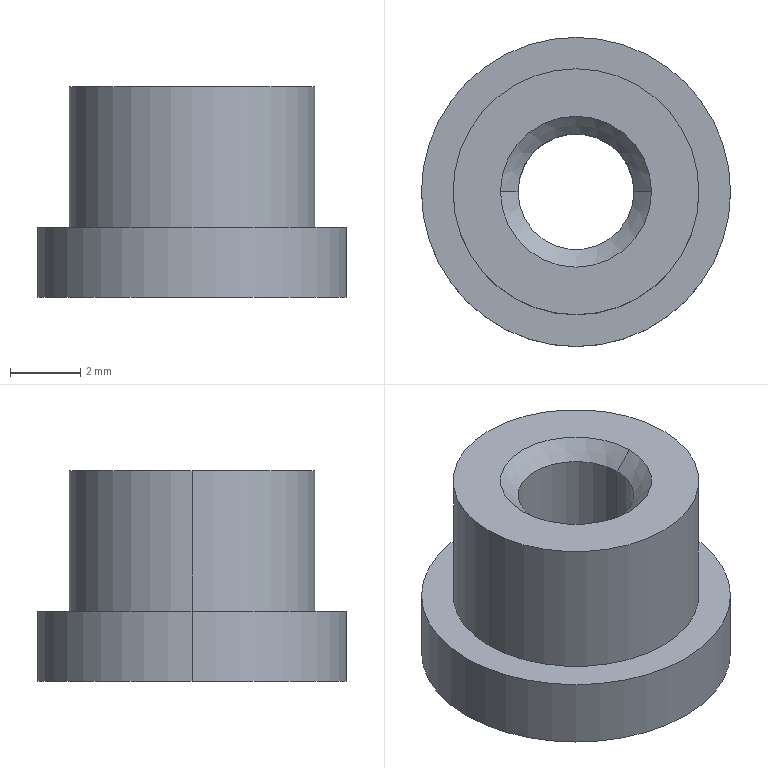Part | STEP file | Ngam kep 11 | 1 solid | 11 faces | box 8.8 x 8.8 x 6 mm | volume 222.836 mm3 | cylinder 6 | plane 3 | cone 2 | commonest cylinder face diameters 3.3 x2 7 x2 8.8 x2
STEP:
#1=CARTESIAN_POINT('',(0.,0.,0.));
#2=DIRECTION('',(0.,0.,1.));
#3=DIRECTION('',(1.,0.,0.));
#4=AXIS2_PLACEMENT_3D('',#1,#2,#3);
#5=CARTESIAN_POINT('',(1.65,0.,2.5));
#6=VERTEX_POINT('',#5);
#7=CARTESIAN_POINT('',(2.15,0.,3.));
#8=VERTEX_POINT('',#7);
#9=CARTESIAN_POINT('',(1.65,0.,2.5));
#10=DIRECTION('',(0.7071,0.,0.7071));
#11=VECTOR('',#10,1.);
#12=LINE('',#9,#11);
#13=CARTESIAN_POINT('',(0.,0.,2.5));
#14=DIRECTION('',(0.,0.,1.));
#15=DIRECTION('',(1.,0.,0.));
#16=AXIS2_PLACEMENT_3D('',#13,#14,#15);
#17=CONICAL_SURFACE('',#16,1.65,0.7854);
#18=CARTESIAN_POINT('',(6.283,0.));
#19=DIRECTION('',(0.,1.));
#20=VECTOR('',#19,1.);
#21=LINE('',#18,#20);
#22=(GEOMETRIC_REPRESENTATION_CONTEXT(2)PARAMETRIC_REPRESENTATION_CONTEXT()REPRESENTATION_CONTEXT('',''));
#23=DEFINITIONAL_REPRESENTATION('',(#21),#22);
#24=PCURVE('',#17,#23);
#25=CARTESIAN_POINT('',(0.,0.,2.5));
#26=DIRECTION('',(0.,0.,1.));
#27=DIRECTION('',(1.,0.,0.));
#28=AXIS2_PLACEMENT_3D('',#25,#26,#27);
#29=CONICAL_SURFACE('',#28,1.65,0.7854);
#30=CARTESIAN_POINT('',(0.,0.));
#31=DIRECTION('',(0.,1.));
#32=VECTOR('',#31,1.);
#33=LINE('',#30,#32);
#34=(GEOMETRIC_REPRESENTATION_CONTEXT(2)PARAMETRIC_REPRESENTATION_CONTEXT()REPRESENTATION_CONTEXT('',''));
#35=DEFINITIONAL_REPRESENTATION('',(#33),#34);
#36=PCURVE('',#29,#35);
#37=SURFACE_CURVE('',#12,(#24,#36),.PCURVE_S1.);
#38=EDGE_CURVE('',#6,#8,#37,.T.);
#39=ORIENTED_EDGE('',*,*,#38,.T.);
#40=CARTESIAN_POINT('',(-2.15,0.,3.));
#41=VERTEX_POINT('',#40);
#42=CARTESIAN_POINT('',(0.,0.,3.));
#43=DIRECTION('',(0.,0.,-1.));
#44=DIRECTION('',(1.,0.,0.));
#45=AXIS2_PLACEMENT_3D('',#42,#43,#44);
#46=CIRCLE('',#45,2.15);
#47=CARTESIAN_POINT('',(6.283,0.5));
#48=DIRECTION('',(-1.,0.));
#49=VECTOR('',#48,1.);
#50=LINE('',#47,#49);
#51=(GEOMETRIC_REPRESENTATION_CONTEXT(2)PARAMETRIC_REPRESENTATION_CONTEXT()REPRESENTATION_CONTEXT('',''));
#52=DEFINITIONAL_REPRESENTATION('',(#50),#51);
#53=PCURVE('',#17,#52);
#54=CARTESIAN_POINT('',(0.,0.,3.));
#55=DIRECTION('',(0.,0.,1.));
#56=DIRECTION('',(1.,0.,0.));
#57=AXIS2_PLACEMENT_3D('',#54,#55,#56);
#58=PLANE('',#57);
#59=CARTESIAN_POINT('',(2.15,0.));
#60=CARTESIAN_POINT('',(2.15,-3.724));
#61=CARTESIAN_POINT('',(-1.075,-1.862));
#62=CARTESIAN_POINT('',(-4.3,0.));
#63=CARTESIAN_POINT('',(-1.075,1.862));
#64=CARTESIAN_POINT('',(2.15,3.724));
#65=CARTESIAN_POINT('',(2.15,0.));
#66=(BOUNDED_CURVE()B_SPLINE_CURVE(2,(#59,#60,#61,#62,#63,#64,#65),.UNSPECIFIED.,.T.,.F.)B_SPLINE_CURVE_WITH_KNOTS((1,2,2,2,2,1),(-2.094,0.,2.094,4.189,6.283,8.378),.UNSPECIFIED.)CURVE()GEOMETRIC_REPRESENTATION_ITEM()RATIONAL_B_SPLINE_CURVE((1.,0.5,1.,0.5,1.,0.5,1.))REPRESENTATION_ITEM(''));
#67=(GEOMETRIC_REPRESENTATION_CONTEXT(2)PARAMETRIC_REPRESENTATION_CONTEXT()REPRESENTATION_CONTEXT('',''));
#68=DEFINITIONAL_REPRESENTATION('',(#66),#67);
#69=PCURVE('',#58,#68);
#70=SURFACE_CURVE('',#46,(#53,#69),.PCURVE_S1.);
#71=EDGE_CURVE('',#8,#41,#70,.T.);
#72=ORIENTED_EDGE('',*,*,#71,.T.);
#73=CARTESIAN_POINT('',(-1.65,0.,2.5));
#74=VERTEX_POINT('',#73);
#75=CARTESIAN_POINT('',(-1.65,0.,2.5));
#76=DIRECTION('',(-0.7071,0.,0.7071));
#77=VECTOR('',#76,1.);
#78=LINE('',#75,#77);
#79=CARTESIAN_POINT('',(3.142,0.));
#80=DIRECTION('',(0.,1.));
#81=VECTOR('',#80,1.);
#82=LINE('',#79,#81);
#83=(GEOMETRIC_REPRESENTATION_CONTEXT(2)PARAMETRIC_REPRESENTATION_CONTEXT()REPRESENTATION_CONTEXT('',''));
#84=DEFINITIONAL_REPRESENTATION('',(#82),#83);
#85=PCURVE('',#17,#84);
#86=CARTESIAN_POINT('',(3.142,0.));
#87=DIRECTION('',(0.,1.));
#88=VECTOR('',#87,1.);
#89=LINE('',#86,#88);
#90=(GEOMETRIC_REPRESENTATION_CONTEXT(2)PARAMETRIC_REPRESENTATION_CONTEXT()REPRESENTATION_CONTEXT('',''));
#91=DEFINITIONAL_REPRESENTATION('',(#89),#90);
#92=PCURVE('',#29,#91);
#93=SURFACE_CURVE('',#78,(#85,#92),.PCURVE_S1.);
#94=EDGE_CURVE('',#74,#41,#93,.T.);
#95=ORIENTED_EDGE('',*,*,#94,.F.);
#96=CARTESIAN_POINT('',(0.,0.,2.5));
#97=DIRECTION('',(0.,0.,1.));
#98=DIRECTION('',(1.,0.,0.));
#99=AXIS2_PLACEMENT_3D('',#96,#97,#98);
#100=CIRCLE('',#99,1.65);
#101=CARTESIAN_POINT('',(0.,0.));
#102=DIRECTION('',(1.,0.));
#103=VECTOR('',#102,1.);
#104=LINE('',#101,#103);
#105=(GEOMETRIC_REPRESENTATION_CONTEXT(2)PARAMETRIC_REPRESENTATION_CONTEXT()REPRESENTATION_CONTEXT('',''));
#106=DEFINITIONAL_REPRESENTATION('',(#104),#105);
#107=PCURVE('',#17,#106);
#108=CARTESIAN_POINT('',(0.,0.,3.));
#109=DIRECTION('',(0.,0.,1.));
#110=DIRECTION('',(1.,0.,0.));
#111=AXIS2_PLACEMENT_3D('',#108,#109,#110);
#112=CYLINDRICAL_SURFACE('',#111,1.65);
#113=CARTESIAN_POINT('',(0.,-0.5));
#114=DIRECTION('',(1.,0.));
#115=VECTOR('',#114,1.);
#116=LINE('',#113,#115);
#117=(GEOMETRIC_REPRESENTATION_CONTEXT(2)PARAMETRIC_REPRESENTATION_CONTEXT()REPRESENTATION_CONTEXT('',''));
#118=DEFINITIONAL_REPRESENTATION('',(#116),#117);
#119=PCURVE('',#112,#118);
#120=SURFACE_CURVE('',#100,(#107,#119),.PCURVE_S1.);
#121=EDGE_CURVE('',#74,#6,#120,.T.);
#122=ORIENTED_EDGE('',*,*,#121,.T.);
#123=EDGE_LOOP('',(#39,#72,#95,#122));
#124=FACE_BOUND('',#123,.F.);
#125=ADVANCED_FACE('',(#124),#17,.F.);
#126=CARTESIAN_POINT('',(1.65,0.,-3.));
#127=VERTEX_POINT('',#126);
#128=CARTESIAN_POINT('',(1.65,0.,3.));
#129=DIRECTION('',(0.,0.,1.));
#130=VECTOR('',#129,1.);
#131=LINE('',#128,#130);
#132=CARTESIAN_POINT('',(6.283,0.));
#133=DIRECTION('',(0.,1.));
#134=VECTOR('',#133,1.);
#135=LINE('',#132,#134);
#136=(GEOMETRIC_REPRESENTATION_CONTEXT(2)PARAMETRIC_REPRESENTATION_CONTEXT()REPRESENTATION_CONTEXT('',''));
#137=DEFINITIONAL_REPRESENTATION('',(#135),#136);
#138=PCURVE('',#112,#137);
#139=CARTESIAN_POINT('',(0.,0.,3.));
#140=DIRECTION('',(0.,0.,1.));
#141=DIRECTION('',(1.,0.,0.));
#142=AXIS2_PLACEMENT_3D('',#139,#140,#141);
#143=CYLINDRICAL_SURFACE('',#142,1.65);
#144=CARTESIAN_POINT('',(0.,0.));
#145=DIRECTION('',(0.,1.));
#146=VECTOR('',#145,1.);
#147=LINE('',#144,#146);
#148=(GEOMETRIC_REPRESENTATION_CONTEXT(2)PARAMETRIC_REPRESENTATION_CONTEXT()REPRESENTATION_CONTEXT('',''));
#149=DEFINITIONAL_REPRESENTATION('',(#147),#148);
#150=PCURVE('',#143,#149);
#151=SURFACE_CURVE('',#131,(#138,#150),.PCURVE_S1.);
#152=EDGE_CURVE('',#127,#6,#151,.T.);
#153=ORIENTED_EDGE('',*,*,#152,.T.);
#154=ORIENTED_EDGE('',*,*,#121,.F.);
#155=CARTESIAN_POINT('',(-1.65,0.,-3.));
#156=VERTEX_POINT('',#155);
#157=CARTESIAN_POINT('',(-1.65,0.,3.));
#158=DIRECTION('',(0.,0.,1.));
#159=VECTOR('',#158,1.);
#160=LINE('',#157,#159);
#161=CARTESIAN_POINT('',(3.142,0.));
#162=DIRECTION('',(0.,1.));
#163=VECTOR('',#162,1.);
#164=LINE('',#161,#163);
#165=(GEOMETRIC_REPRESENTATION_CONTEXT(2)PARAMETRIC_REPRESENTATION_CONTEXT()REPRESENTATION_CONTEXT('',''));
#166=DEFINITIONAL_REPRESENTATION('',(#164),#165);
#167=PCURVE('',#112,#166);
#168=CARTESIAN_POINT('',(3.142,0.));
#169=DIRECTION('',(0.,1.));
#170=VECTOR('',#169,1.);
#171=LINE('',#168,#170);
#172=(GEOMETRIC_REPRESENTATION_CONTEXT(2)PARAMETRIC_REPRESENTATION_CONTEXT()REPRESENTATION_CONTEXT('',''));
#173=DEFINITIONAL_REPRESENTATION('',(#171),#172);
#174=PCURVE('',#143,#173);
#175=SURFACE_CURVE('',#160,(#167,#174),.PCURVE_S1.);
#176=EDGE_CURVE('',#156,#74,#175,.T.);
#177=ORIENTED_EDGE('',*,*,#176,.F.);
#178=CARTESIAN_POINT('',(0.,0.,-3.));
#179=DIRECTION('',(0.,0.,1.));
#180=DIRECTION('',(1.,0.,0.));
#181=AXIS2_PLACEMENT_3D('',#178,#179,#180);
#182=CIRCLE('',#181,1.65);
#183=CARTESIAN_POINT('',(0.,-6.));
#184=DIRECTION('',(1.,0.));
#185=VECTOR('',#184,1.);
#186=LINE('',#183,#185);
#187=(GEOMETRIC_REPRESENTATION_CONTEXT(2)PARAMETRIC_REPRESENTATION_CONTEXT()REPRESENTATION_CONTEXT('',''));
#188=DEFINITIONAL_REPRESENTATION('',(#186),#187);
#189=PCURVE('',#112,#188);
#190=CARTESIAN_POINT('',(0.,0.,-3.));
#191=DIRECTION('',(0.,0.,1.));
#192=DIRECTION('',(1.,0.,0.));
#193=AXIS2_PLACEMENT_3D('',#190,#191,#192);
#194=PLANE('',#193);
#195=CARTESIAN_POINT('',(0.,0.));
#196=DIRECTION('',(1.,0.));
#197=AXIS2_PLACEMENT_2D('',#195,#196);
#198=CIRCLE('',#197,1.65);
#199=(GEOMETRIC_REPRESENTATION_CONTEXT(2)PARAMETRIC_REPRESENTATION_CONTEXT()REPRESENTATION_CONTEXT('',''));
#200=DEFINITIONAL_REPRESENTATION('',(#198),#199);
#201=PCURVE('',#194,#200);
#202=SURFACE_CURVE('',#182,(#189,#201),.PCURVE_S1.);
#203=EDGE_CURVE('',#156,#127,#202,.T.);
#204=ORIENTED_EDGE('',*,*,#203,.T.);
#205=EDGE_LOOP('',(#153,#154,#177,#204));
#206=FACE_BOUND('',#205,.F.);
#207=ADVANCED_FACE('',(#206),#112,.F.);
#208=CARTESIAN_POINT('',(4.4,0.,-1.));
#209=VERTEX_POINT('',#208);
#210=CARTESIAN_POINT('',(-4.4,0.,-1.));
#211=VERTEX_POINT('',#210);
#212=CARTESIAN_POINT('',(0.,0.,-1.));
#213=DIRECTION('',(0.,0.,1.));
#214=DIRECTION('',(1.,0.,0.));
#215=AXIS2_PLACEMENT_3D('',#212,#213,#214);
#216=CIRCLE('',#215,4.4);
#217=CARTESIAN_POINT('',(0.,0.,-1.));
#218=DIRECTION('',(0.,0.,-1.));
#219=DIRECTION('',(-1.,0.,0.));
#220=AXIS2_PLACEMENT_3D('',#217,#218,#219);
#221=CYLINDRICAL_SURFACE('',#220,4.4);
#222=CARTESIAN_POINT('',(3.142,0.));
#223=DIRECTION('',(-1.,0.));
#224=VECTOR('',#223,1.);
#225=LINE('',#222,#224);
#226=(GEOMETRIC_REPRESENTATION_CONTEXT(2)PARAMETRIC_REPRESENTATION_CONTEXT()REPRESENTATION_CONTEXT('',''));
#227=DEFINITIONAL_REPRESENTATION('',(#225),#226);
#228=PCURVE('',#221,#227);
#229=CARTESIAN_POINT('',(0.,0.,-1.));
#230=DIRECTION('',(0.,0.,1.));
#231=DIRECTION('',(1.,0.,0.));
#232=AXIS2_PLACEMENT_3D('',#229,#230,#231);
#233=PLANE('',#232);
#234=CARTESIAN_POINT('',(0.,0.));
#235=DIRECTION('',(1.,0.));
#236=AXIS2_PLACEMENT_2D('',#234,#235);
#237=CIRCLE('',#236,4.4);
#238=(GEOMETRIC_REPRESENTATION_CONTEXT(2)PARAMETRIC_REPRESENTATION_CONTEXT()REPRESENTATION_CONTEXT('',''));
#239=DEFINITIONAL_REPRESENTATION('',(#237),#238);
#240=PCURVE('',#233,#239);
#241=SURFACE_CURVE('',#216,(#228,#240),.PCURVE_S1.);
#242=EDGE_CURVE('',#209,#211,#241,.T.);
#243=ORIENTED_EDGE('',*,*,#242,.F.);
#244=CARTESIAN_POINT('',(4.4,0.,-3.));
#245=VERTEX_POINT('',#244);
#246=CARTESIAN_POINT('',(4.4,0.,-1.));
#247=DIRECTION('',(0.,0.,-1.));
#248=VECTOR('',#247,1.);
#249=LINE('',#246,#248);
#250=CARTESIAN_POINT('',(3.142,0.));
#251=DIRECTION('',(0.,1.));
#252=VECTOR('',#251,1.);
#253=LINE('',#250,#252);
#254=(GEOMETRIC_REPRESENTATION_CONTEXT(2)PARAMETRIC_REPRESENTATION_CONTEXT()REPRESENTATION_CONTEXT('',''));
#255=DEFINITIONAL_REPRESENTATION('',(#253),#254);
#256=PCURVE('',#221,#255);
#257=CARTESIAN_POINT('',(0.,0.,-1.));
#258=DIRECTION('',(0.,0.,-1.));
#259=DIRECTION('',(-1.,0.,0.));
#260=AXIS2_PLACEMENT_3D('',#257,#258,#259);
#261=CYLINDRICAL_SURFACE('',#260,4.4);
#262=CARTESIAN_POINT('',(3.142,0.));
#263=DIRECTION('',(0.,1.));
#264=VECTOR('',#263,1.);
#265=LINE('',#262,#264);
#266=(GEOMETRIC_REPRESENTATION_CONTEXT(2)PARAMETRIC_REPRESENTATION_CONTEXT()REPRESENTATION_CONTEXT('',''));
#267=DEFINITIONAL_REPRESENTATION('',(#265),#266);
#268=PCURVE('',#261,#267);
#269=SURFACE_CURVE('',#249,(#256,#268),.PCURVE_S1.);
#270=EDGE_CURVE('',#209,#245,#269,.T.);
#271=ORIENTED_EDGE('',*,*,#270,.T.);
#272=CARTESIAN_POINT('',(-4.4,0.,-3.));
#273=VERTEX_POINT('',#272);
#274=CARTESIAN_POINT('',(0.,0.,-3.));
#275=DIRECTION('',(0.,0.,1.));
#276=DIRECTION('',(1.,0.,0.));
#277=AXIS2_PLACEMENT_3D('',#274,#275,#276);
#278=CIRCLE('',#277,4.4);
#279=CARTESIAN_POINT('',(3.142,2.));
#280=DIRECTION('',(-1.,0.));
#281=VECTOR('',#280,1.);
#282=LINE('',#279,#281);
#283=(GEOMETRIC_REPRESENTATION_CONTEXT(2)PARAMETRIC_REPRESENTATION_CONTEXT()REPRESENTATION_CONTEXT('',''));
#284=DEFINITIONAL_REPRESENTATION('',(#282),#283);
#285=PCURVE('',#221,#284);
#286=CARTESIAN_POINT('',(0.,0.));
#287=DIRECTION('',(1.,0.));
#288=AXIS2_PLACEMENT_2D('',#286,#287);
#289=CIRCLE('',#288,4.4);
#290=(GEOMETRIC_REPRESENTATION_CONTEXT(2)PARAMETRIC_REPRESENTATION_CONTEXT()REPRESENTATION_CONTEXT('',''));
#291=DEFINITIONAL_REPRESENTATION('',(#289),#290);
#292=PCURVE('',#194,#291);
#293=SURFACE_CURVE('',#278,(#285,#292),.PCURVE_S1.);
#294=EDGE_CURVE('',#245,#273,#293,.T.);
#295=ORIENTED_EDGE('',*,*,#294,.T.);
#296=CARTESIAN_POINT('',(-4.4,0.,-1.));
#297=DIRECTION('',(0.,0.,-1.));
#298=VECTOR('',#297,1.);
#299=LINE('',#296,#298);
#300=CARTESIAN_POINT('',(0.,0.));
#301=DIRECTION('',(0.,1.));
#302=VECTOR('',#301,1.);
#303=LINE('',#300,#302);
#304=(GEOMETRIC_REPRESENTATION_CONTEXT(2)PARAMETRIC_REPRESENTATION_CONTEXT()REPRESENTATION_CONTEXT('',''));
#305=DEFINITIONAL_REPRESENTATION('',(#303),#304);
#306=PCURVE('',#221,#305);
#307=CARTESIAN_POINT('',(6.283,0.));
#308=DIRECTION('',(0.,1.));
#309=VECTOR('',#308,1.);
#310=LINE('',#307,#309);
#311=(GEOMETRIC_REPRESENTATION_CONTEXT(2)PARAMETRIC_REPRESENTATION_CONTEXT()REPRESENTATION_CONTEXT('',''));
#312=DEFINITIONAL_REPRESENTATION('',(#310),#311);
#313=PCURVE('',#261,#312);
#314=SURFACE_CURVE('',#299,(#306,#313),.PCURVE_S1.);
#315=EDGE_CURVE('',#211,#273,#314,.T.);
#316=ORIENTED_EDGE('',*,*,#315,.F.);
#317=EDGE_LOOP('',(#243,#271,#295,#316));
#318=FACE_BOUND('',#317,.T.);
#319=ADVANCED_FACE('',(#318),#221,.T.);
#320=CARTESIAN_POINT('',(3.5,0.,3.));
#321=VERTEX_POINT('',#320);
#322=CARTESIAN_POINT('',(-3.5,0.,3.));
#323=VERTEX_POINT('',#322);
#324=CARTESIAN_POINT('',(0.,0.,3.));
#325=DIRECTION('',(0.,0.,1.));
#326=DIRECTION('',(1.,0.,0.));
#327=AXIS2_PLACEMENT_3D('',#324,#325,#326);
#328=CIRCLE('',#327,3.5);
#329=CARTESIAN_POINT('',(0.,0.,3.));
#330=DIRECTION('',(0.,0.,-1.));
#331=DIRECTION('',(-1.,0.,0.));
#332=AXIS2_PLACEMENT_3D('',#329,#330,#331);
#333=CYLINDRICAL_SURFACE('',#332,3.5);
#334=CARTESIAN_POINT('',(3.142,0.));
#335=DIRECTION('',(-1.,0.));
#336=VECTOR('',#335,1.);
#337=LINE('',#334,#336);
#338=(GEOMETRIC_REPRESENTATION_CONTEXT(2)PARAMETRIC_REPRESENTATION_CONTEXT()REPRESENTATION_CONTEXT('',''));
#339=DEFINITIONAL_REPRESENTATION('',(#337),#338);
#340=PCURVE('',#333,#339);
#341=CARTESIAN_POINT('',(0.,0.));
#342=DIRECTION('',(1.,0.));
#343=AXIS2_PLACEMENT_2D('',#341,#342);
#344=CIRCLE('',#343,3.5);
#345=(GEOMETRIC_REPRESENTATION_CONTEXT(2)PARAMETRIC_REPRESENTATION_CONTEXT()REPRESENTATION_CONTEXT('',''));
#346=DEFINITIONAL_REPRESENTATION('',(#344),#345);
#347=PCURVE('',#58,#346);
#348=SURFACE_CURVE('',#328,(#340,#347),.PCURVE_S1.);
#349=EDGE_CURVE('',#321,#323,#348,.T.);
#350=ORIENTED_EDGE('',*,*,#349,.F.);
#351=CARTESIAN_POINT('',(3.5,0.,-1.));
#352=VERTEX_POINT('',#351);
#353=CARTESIAN_POINT('',(3.5,0.,3.));
#354=DIRECTION('',(0.,0.,-1.));
#355=VECTOR('',#354,1.);
#356=LINE('',#353,#355);
#357=CARTESIAN_POINT('',(3.142,0.));
#358=DIRECTION('',(0.,1.));
#359=VECTOR('',#358,1.);
#360=LINE('',#357,#359);
#361=(GEOMETRIC_REPRESENTATION_CONTEXT(2)PARAMETRIC_REPRESENTATION_CONTEXT()REPRESENTATION_CONTEXT('',''));
#362=DEFINITIONAL_REPRESENTATION('',(#360),#361);
#363=PCURVE('',#333,#362);
#364=CARTESIAN_POINT('',(0.,0.,3.));
#365=DIRECTION('',(0.,0.,-1.));
#366=DIRECTION('',(-1.,0.,0.));
#367=AXIS2_PLACEMENT_3D('',#364,#365,#366);
#368=CYLINDRICAL_SURFACE('',#367,3.5);
#369=CARTESIAN_POINT('',(3.142,0.));
#370=DIRECTION('',(0.,1.));
#371=VECTOR('',#370,1.);
#372=LINE('',#369,#371);
#373=(GEOMETRIC_REPRESENTATION_CONTEXT(2)PARAMETRIC_REPRESENTATION_CONTEXT()REPRESENTATION_CONTEXT('',''));
#374=DEFINITIONAL_REPRESENTATION('',(#372),#373);
#375=PCURVE('',#368,#374);
#376=SURFACE_CURVE('',#356,(#363,#375),.PCURVE_S1.);
#377=EDGE_CURVE('',#321,#352,#376,.T.);
#378=ORIENTED_EDGE('',*,*,#377,.T.);
#379=CARTESIAN_POINT('',(-3.5,0.,-1.));
#380=VERTEX_POINT('',#379);
#381=CARTESIAN_POINT('',(0.,0.,-1.));
#382=DIRECTION('',(0.,0.,1.));
#383=DIRECTION('',(1.,0.,0.));
#384=AXIS2_PLACEMENT_3D('',#381,#382,#383);
#385=CIRCLE('',#384,3.5);
#386=CARTESIAN_POINT('',(3.142,4.));
#387=DIRECTION('',(-1.,0.));
#388=VECTOR('',#387,1.);
#389=LINE('',#386,#388);
#390=(GEOMETRIC_REPRESENTATION_CONTEXT(2)PARAMETRIC_REPRESENTATION_CONTEXT()REPRESENTATION_CONTEXT('',''));
#391=DEFINITIONAL_REPRESENTATION('',(#389),#390);
#392=PCURVE('',#333,#391);
#393=CARTESIAN_POINT('',(0.,0.));
#394=DIRECTION('',(1.,0.));
#395=AXIS2_PLACEMENT_2D('',#393,#394);
#396=CIRCLE('',#395,3.5);
#397=(GEOMETRIC_REPRESENTATION_CONTEXT(2)PARAMETRIC_REPRESENTATION_CONTEXT()REPRESENTATION_CONTEXT('',''));
#398=DEFINITIONAL_REPRESENTATION('',(#396),#397);
#399=PCURVE('',#233,#398);
#400=SURFACE_CURVE('',#385,(#392,#399),.PCURVE_S1.);
#401=EDGE_CURVE('',#352,#380,#400,.T.);
#402=ORIENTED_EDGE('',*,*,#401,.T.);
#403=CARTESIAN_POINT('',(-3.5,0.,3.));
#404=DIRECTION('',(0.,0.,-1.));
#405=VECTOR('',#404,1.);
#406=LINE('',#403,#405);
#407=CARTESIAN_POINT('',(0.,0.));
#408=DIRECTION('',(0.,1.));
#409=VECTOR('',#408,1.);
#410=LINE('',#407,#409);
#411=(GEOMETRIC_REPRESENTATION_CONTEXT(2)PARAMETRIC_REPRESENTATION_CONTEXT()REPRESENTATION_CONTEXT('',''));
#412=DEFINITIONAL_REPRESENTATION('',(#410),#411);
#413=PCURVE('',#333,#412);
#414=CARTESIAN_POINT('',(6.283,0.));
#415=DIRECTION('',(0.,1.));
#416=VECTOR('',#415,1.);
#417=LINE('',#414,#416);
#418=(GEOMETRIC_REPRESENTATION_CONTEXT(2)PARAMETRIC_REPRESENTATION_CONTEXT()REPRESENTATION_CONTEXT('',''));
#419=DEFINITIONAL_REPRESENTATION('',(#417),#418);
#420=PCURVE('',#368,#419);
#421=SURFACE_CURVE('',#406,(#413,#420),.PCURVE_S1.);
#422=EDGE_CURVE('',#323,#380,#421,.T.);
#423=ORIENTED_EDGE('',*,*,#422,.F.);
#424=EDGE_LOOP('',(#350,#378,#402,#423));
#425=FACE_BOUND('',#424,.T.);
#426=ADVANCED_FACE('',(#425),#333,.T.);
#427=ORIENTED_EDGE('',*,*,#377,.F.);
#428=CARTESIAN_POINT('',(0.,0.,3.));
#429=DIRECTION('',(0.,0.,1.));
#430=DIRECTION('',(1.,0.,0.));
#431=AXIS2_PLACEMENT_3D('',#428,#429,#430);
#432=CIRCLE('',#431,3.5);
#433=CARTESIAN_POINT('',(9.425,0.));
#434=DIRECTION('',(-1.,0.));
#435=VECTOR('',#434,1.);
#436=LINE('',#433,#435);
#437=(GEOMETRIC_REPRESENTATION_CONTEXT(2)PARAMETRIC_REPRESENTATION_CONTEXT()REPRESENTATION_CONTEXT('',''));
#438=DEFINITIONAL_REPRESENTATION('',(#436),#437);
#439=PCURVE('',#368,#438);
#440=CARTESIAN_POINT('',(0.,0.));
#441=DIRECTION('',(1.,0.));
#442=AXIS2_PLACEMENT_2D('',#440,#441);
#443=CIRCLE('',#442,3.5);
#444=(GEOMETRIC_REPRESENTATION_CONTEXT(2)PARAMETRIC_REPRESENTATION_CONTEXT()REPRESENTATION_CONTEXT('',''));
#445=DEFINITIONAL_REPRESENTATION('',(#443),#444);
#446=PCURVE('',#58,#445);
#447=SURFACE_CURVE('',#432,(#439,#446),.PCURVE_S1.);
#448=EDGE_CURVE('',#323,#321,#447,.T.);
#449=ORIENTED_EDGE('',*,*,#448,.F.);
#450=ORIENTED_EDGE('',*,*,#422,.T.);
#451=CARTESIAN_POINT('',(0.,0.,-1.));
#452=DIRECTION('',(0.,0.,1.));
#453=DIRECTION('',(1.,0.,0.));
#454=AXIS2_PLACEMENT_3D('',#451,#452,#453);
#455=CIRCLE('',#454,3.5);
#456=CARTESIAN_POINT('',(9.425,4.));
#457=DIRECTION('',(-1.,0.));
#458=VECTOR('',#457,1.);
#459=LINE('',#456,#458);
#460=(GEOMETRIC_REPRESENTATION_CONTEXT(2)PARAMETRIC_REPRESENTATION_CONTEXT()REPRESENTATION_CONTEXT('',''));
#461=DEFINITIONAL_REPRESENTATION('',(#459),#460);
#462=PCURVE('',#368,#461);
#463=CARTESIAN_POINT('',(0.,0.));
#464=DIRECTION('',(1.,0.));
#465=AXIS2_PLACEMENT_2D('',#463,#464);
#466=CIRCLE('',#465,3.5);
#467=(GEOMETRIC_REPRESENTATION_CONTEXT(2)PARAMETRIC_REPRESENTATION_CONTEXT()REPRESENTATION_CONTEXT('',''));
#468=DEFINITIONAL_REPRESENTATION('',(#466),#467);
#469=PCURVE('',#233,#468);
#470=SURFACE_CURVE('',#455,(#462,#469),.PCURVE_S1.);
#471=EDGE_CURVE('',#380,#352,#470,.T.);
#472=ORIENTED_EDGE('',*,*,#471,.T.);
#473=EDGE_LOOP('',(#427,#449,#450,#472));
#474=FACE_BOUND('',#473,.T.);
#475=ADVANCED_FACE('',(#474),#368,.T.);
#476=ORIENTED_EDGE('',*,*,#71,.T.);
#477=CARTESIAN_POINT('',(0.,0.,3.));
#478=DIRECTION('',(0.,0.,-1.));
#479=DIRECTION('',(1.,0.,0.));
#480=AXIS2_PLACEMENT_3D('',#477,#478,#479);
#481=CIRCLE('',#480,2.15);
#482=CARTESIAN_POINT('',(2.15,0.));
#483=CARTESIAN_POINT('',(2.15,-3.724));
#484=CARTESIAN_POINT('',(-1.075,-1.862));
#485=CARTESIAN_POINT('',(-4.3,0.));
#486=CARTESIAN_POINT('',(-1.075,1.862));
#487=CARTESIAN_POINT('',(2.15,3.724));
#488=CARTESIAN_POINT('',(2.15,0.));
#489=(BOUNDED_CURVE()B_SPLINE_CURVE(2,(#482,#483,#484,#485,#486,#487,#488),.UNSPECIFIED.,.T.,.F.)B_SPLINE_CURVE_WITH_KNOTS((1,2,2,2,2,1),(-2.094,0.,2.094,4.189,6.283,8.378),.UNSPECIFIED.)CURVE()GEOMETRIC_REPRESENTATION_ITEM()RATIONAL_B_SPLINE_CURVE((1.,0.5,1.,0.5,1.,0.5,1.))REPRESENTATION_ITEM(''));
#490=(GEOMETRIC_REPRESENTATION_CONTEXT(2)PARAMETRIC_REPRESENTATION_CONTEXT()REPRESENTATION_CONTEXT('',''));
#491=DEFINITIONAL_REPRESENTATION('',(#489),#490);
#492=PCURVE('',#58,#491);
#493=CARTESIAN_POINT('',(6.283,0.5));
#494=DIRECTION('',(-1.,0.));
#495=VECTOR('',#494,1.);
#496=LINE('',#493,#495);
#497=(GEOMETRIC_REPRESENTATION_CONTEXT(2)PARAMETRIC_REPRESENTATION_CONTEXT()REPRESENTATION_CONTEXT('',''));
#498=DEFINITIONAL_REPRESENTATION('',(#496),#497);
#499=PCURVE('',#29,#498);
#500=SURFACE_CURVE('',#481,(#492,#499),.PCURVE_S1.);
#501=EDGE_CURVE('',#41,#8,#500,.T.);
#502=ORIENTED_EDGE('',*,*,#501,.T.);
#503=EDGE_LOOP('',(#476,#502));
#504=FACE_BOUND('',#503,.T.);
#505=ORIENTED_EDGE('',*,*,#448,.T.);
#506=ORIENTED_EDGE('',*,*,#349,.T.);
#507=EDGE_LOOP('',(#505,#506));
#508=FACE_BOUND('',#507,.T.);
#509=ADVANCED_FACE('',(#504,#508),#58,.T.);
#510=CARTESIAN_POINT('',(0.,0.,-1.));
#511=DIRECTION('',(0.,0.,1.));
#512=DIRECTION('',(1.,0.,0.));
#513=AXIS2_PLACEMENT_3D('',#510,#511,#512);
#514=CIRCLE('',#513,4.4);
#515=CARTESIAN_POINT('',(0.,0.));
#516=DIRECTION('',(1.,0.));
#517=AXIS2_PLACEMENT_2D('',#515,#516);
#518=CIRCLE('',#517,4.4);
#519=(GEOMETRIC_REPRESENTATION_CONTEXT(2)PARAMETRIC_REPRESENTATION_CONTEXT()REPRESENTATION_CONTEXT('',''));
#520=DEFINITIONAL_REPRESENTATION('',(#518),#519);
#521=PCURVE('',#233,#520);
#522=CARTESIAN_POINT('',(9.425,0.));
#523=DIRECTION('',(-1.,0.));
#524=VECTOR('',#523,1.);
#525=LINE('',#522,#524);
#526=(GEOMETRIC_REPRESENTATION_CONTEXT(2)PARAMETRIC_REPRESENTATION_CONTEXT()REPRESENTATION_CONTEXT('',''));
#527=DEFINITIONAL_REPRESENTATION('',(#525),#526);
#528=PCURVE('',#261,#527);
#529=SURFACE_CURVE('',#514,(#521,#528),.PCURVE_S1.);
#530=EDGE_CURVE('',#211,#209,#529,.T.);
#531=ORIENTED_EDGE('',*,*,#530,.T.);
#532=ORIENTED_EDGE('',*,*,#242,.T.);
#533=EDGE_LOOP('',(#531,#532));
#534=FACE_BOUND('',#533,.T.);
#535=ORIENTED_EDGE('',*,*,#471,.F.);
#536=ORIENTED_EDGE('',*,*,#401,.F.);
#537=EDGE_LOOP('',(#535,#536));
#538=FACE_BOUND('',#537,.T.);
#539=ADVANCED_FACE('',(#534,#538),#233,.T.);
#540=ORIENTED_EDGE('',*,*,#270,.F.);
#541=ORIENTED_EDGE('',*,*,#530,.F.);
#542=ORIENTED_EDGE('',*,*,#315,.T.);
#543=CARTESIAN_POINT('',(0.,0.,-3.));
#544=DIRECTION('',(0.,0.,1.));
#545=DIRECTION('',(1.,0.,0.));
#546=AXIS2_PLACEMENT_3D('',#543,#544,#545);
#547=CIRCLE('',#546,4.4);
#548=CARTESIAN_POINT('',(9.425,2.));
#549=DIRECTION('',(-1.,0.));
#550=VECTOR('',#549,1.);
#551=LINE('',#548,#550);
#552=(GEOMETRIC_REPRESENTATION_CONTEXT(2)PARAMETRIC_REPRESENTATION_CONTEXT()REPRESENTATION_CONTEXT('',''));
#553=DEFINITIONAL_REPRESENTATION('',(#551),#552);
#554=PCURVE('',#261,#553);
#555=CARTESIAN_POINT('',(0.,0.));
#556=DIRECTION('',(1.,0.));
#557=AXIS2_PLACEMENT_2D('',#555,#556);
#558=CIRCLE('',#557,4.4);
#559=(GEOMETRIC_REPRESENTATION_CONTEXT(2)PARAMETRIC_REPRESENTATION_CONTEXT()REPRESENTATION_CONTEXT('',''));
#560=DEFINITIONAL_REPRESENTATION('',(#558),#559);
#561=PCURVE('',#194,#560);
#562=SURFACE_CURVE('',#547,(#554,#561),.PCURVE_S1.);
#563=EDGE_CURVE('',#273,#245,#562,.T.);
#564=ORIENTED_EDGE('',*,*,#563,.T.);
#565=EDGE_LOOP('',(#540,#541,#542,#564));
#566=FACE_BOUND('',#565,.T.);
#567=ADVANCED_FACE('',(#566),#261,.T.);
#568=CARTESIAN_POINT('',(0.,0.,-3.));
#569=DIRECTION('',(0.,0.,1.));
#570=DIRECTION('',(1.,0.,0.));
#571=AXIS2_PLACEMENT_3D('',#568,#569,#570);
#572=CIRCLE('',#571,1.65);
#573=CARTESIAN_POINT('',(0.,0.));
#574=DIRECTION('',(1.,0.));
#575=AXIS2_PLACEMENT_2D('',#573,#574);
#576=CIRCLE('',#575,1.65);
#577=(GEOMETRIC_REPRESENTATION_CONTEXT(2)PARAMETRIC_REPRESENTATION_CONTEXT()REPRESENTATION_CONTEXT('',''));
#578=DEFINITIONAL_REPRESENTATION('',(#576),#577);
#579=PCURVE('',#194,#578);
#580=CARTESIAN_POINT('',(0.,-6.));
#581=DIRECTION('',(1.,0.));
#582=VECTOR('',#581,1.);
#583=LINE('',#580,#582);
#584=(GEOMETRIC_REPRESENTATION_CONTEXT(2)PARAMETRIC_REPRESENTATION_CONTEXT()REPRESENTATION_CONTEXT('',''));
#585=DEFINITIONAL_REPRESENTATION('',(#583),#584);
#586=PCURVE('',#143,#585);
#587=SURFACE_CURVE('',#572,(#579,#586),.PCURVE_S1.);
#588=EDGE_CURVE('',#127,#156,#587,.T.);
#589=ORIENTED_EDGE('',*,*,#588,.T.);
#590=ORIENTED_EDGE('',*,*,#203,.T.);
#591=EDGE_LOOP('',(#589,#590));
#592=FACE_BOUND('',#591,.T.);
#593=ORIENTED_EDGE('',*,*,#563,.F.);
#594=ORIENTED_EDGE('',*,*,#294,.F.);
#595=EDGE_LOOP('',(#593,#594));
#596=FACE_BOUND('',#595,.T.);
#597=ADVANCED_FACE('',(#592,#596),#194,.F.);
#598=CARTESIAN_POINT('',(0.,0.,2.5));
#599=DIRECTION('',(0.,0.,1.));
#600=DIRECTION('',(1.,0.,0.));
#601=AXIS2_PLACEMENT_3D('',#598,#599,#600);
#602=CIRCLE('',#601,1.65);
#603=CARTESIAN_POINT('',(0.,-0.5));
#604=DIRECTION('',(1.,0.));
#605=VECTOR('',#604,1.);
#606=LINE('',#603,#605);
#607=(GEOMETRIC_REPRESENTATION_CONTEXT(2)PARAMETRIC_REPRESENTATION_CONTEXT()REPRESENTATION_CONTEXT('',''));
#608=DEFINITIONAL_REPRESENTATION('',(#606),#607);
#609=PCURVE('',#143,#608);
#610=CARTESIAN_POINT('',(0.,0.));
#611=DIRECTION('',(1.,0.));
#612=VECTOR('',#611,1.);
#613=LINE('',#610,#612);
#614=(GEOMETRIC_REPRESENTATION_CONTEXT(2)PARAMETRIC_REPRESENTATION_CONTEXT()REPRESENTATION_CONTEXT('',''));
#615=DEFINITIONAL_REPRESENTATION('',(#613),#614);
#616=PCURVE('',#29,#615);
#617=SURFACE_CURVE('',#602,(#609,#616),.PCURVE_S1.);
#618=EDGE_CURVE('',#6,#74,#617,.T.);
#619=ORIENTED_EDGE('',*,*,#618,.F.);
#620=ORIENTED_EDGE('',*,*,#152,.F.);
#621=ORIENTED_EDGE('',*,*,#588,.T.);
#622=ORIENTED_EDGE('',*,*,#176,.T.);
#623=EDGE_LOOP('',(#619,#620,#621,#622));
#624=FACE_BOUND('',#623,.F.);
#625=ADVANCED_FACE('',(#624),#143,.F.);
#626=ORIENTED_EDGE('',*,*,#501,.T.);
#627=ORIENTED_EDGE('',*,*,#38,.F.);
#628=ORIENTED_EDGE('',*,*,#618,.T.);
#629=ORIENTED_EDGE('',*,*,#94,.T.);
#630=EDGE_LOOP('',(#626,#627,#628,#629));
#631=FACE_BOUND('',#630,.F.);
#632=ADVANCED_FACE('',(#631),#29,.F.);
#633=CLOSED_SHELL('',(#125,#207,#319,#426,#475,#509,#539,#567,#597,#625,#632));
#634=MANIFOLD_SOLID_BREP('',#633);
#635=(LENGTH_UNIT()NAMED_UNIT(*)SI_UNIT(.MILLI.,.METRE.));
#636=UNCERTAINTY_MEASURE_WITH_UNIT(LENGTH_MEASURE(0.0000001),#635,'','');
#637=(NAMED_UNIT(*)PLANE_ANGLE_UNIT()SI_UNIT($,.RADIAN.));
#638=(NAMED_UNIT(*)SI_UNIT($,.STERADIAN.)SOLID_ANGLE_UNIT());
#639=(GEOMETRIC_REPRESENTATION_CONTEXT(3)GLOBAL_UNCERTAINTY_ASSIGNED_CONTEXT((#636))GLOBAL_UNIT_ASSIGNED_CONTEXT((#635,#637,#638))REPRESENTATION_CONTEXT('',''));
#640=ADVANCED_BREP_SHAPE_REPRESENTATION('',(#4,#634),#639);